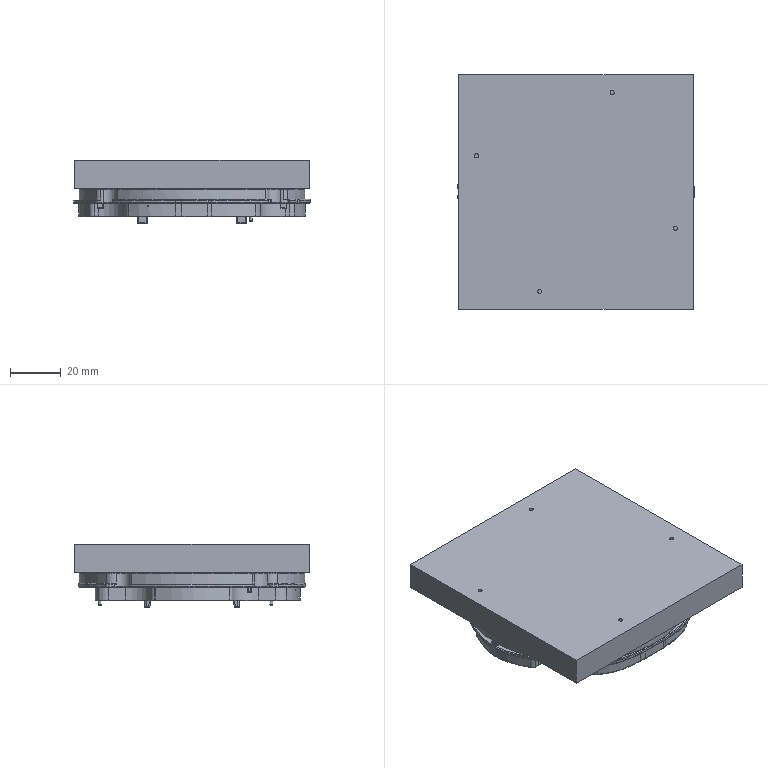NC program | NX | posted with a generic post | part box 92.935 x 92.1 x 24.829 mm
Lines 5782 to 7422 of 7643, first 1500 of 1619 lines:
(PLANAR_MILL_2_COPY , TOOL : D8-25-D8-60-3T-FINISH)
N11508 T16 M6
N11510 G53
N11512 G17 G0 G90 X-29.055 Y-31.838 S3500 M3
N11514 G43 Z21. H16
N11516 Z2.
N11518 G94 G1 Z0. F800.
N11520 G3 X-29.055 Y-29.009 R2.
N11522 G1 X-44.744 Y-13.321
N11524 G2 X-47.69 Y-7.539 R10.5
N11526 X-47.69 Y7.563 R48.25
N11528 X-44.744 Y13.345 R10.5
N11530 G1 X-13.367 Y44.721
N11532 G2 X-7.586 Y47.667 R10.5
N11534 X7.517 Y47.667 R48.25
N11536 X13.298 Y44.721 R10.5
N11538 G1 X18.008 Y40.012
N11540 X23.489
N11542 G2 X30.689 Y32.812 R7.2
N11544 G1 Y27.331
N11546 X44.675 Y13.345
N11548 G2 X47.621 Y7.563 R10.5
N11550 X47.621 Y-7.539 R48.25
N11552 X44.675 Y-13.321 R10.5
N11554 G1 X13.298 Y-44.697
N11556 G2 X7.517 Y-47.643 R10.5
N11558 X-7.586 Y-47.643 R48.25
N11560 X-13.367 Y-44.697 R10.5
N11562 G1 X-29.055 Y-29.009
N11564 G3 X-31.884 Y-29.009 R2.
N11566 G1 X-26.793 Y-29.575
N11568 G3 X-26.793 Y-26.746 R2.
N11570 G1 X-42.481 Y-11.058
N11572 G2 X-44.529 Y-7.039 R7.3
N11574 X-44.529 Y7.063 R45.05
N11576 X-42.481 Y11.082 R7.3
N11578 G1 X-11.104 Y42.459
N11580 G2 X-7.085 Y44.507 R7.3
N11582 X7.016 Y44.507 R45.05
N11584 X11.036 Y42.459 R7.3
N11586 G1 X15.892 Y37.603
N11588 G3 X17.801 Y36.812 R2.7
N11590 G1 X23.489
N11592 G2 X27.489 Y32.812 R4.
N11594 G1 Y27.124
N11596 G3 X28.279 Y25.215 R2.7
N11598 G1 X42.412 Y11.082
N11600 G2 X44.461 Y7.063 R7.3
N11602 X44.461 Y-7.039 R45.05
N11604 X42.412 Y-11.058 R7.3
N11606 G1 X11.036 Y-42.435
N11608 G2 X7.016 Y-44.483 R7.3
N11610 X-7.085 Y-44.483 R45.05
N11612 X-11.104 Y-42.435 R7.3
N11614 G1 X-26.793 Y-26.746
N11616 G3 X-29.621 Y-26.746 R2.
N11618 G1 X-31.884 Y-29.009
N11620 Z2.
N11622 G0 Z21.
(CAVITY_MILL , TOOL : D8-25-D8-60-3T-FINISH)
N11624 X1.671 Y-50.455
N11626 Z-14.
N11628 G1 Z-16.
N11630 G3 X-0.324 Y-48.45 R2.
N11632 G2 X-4.38 Y-48.368 R115.196
N11634 X-10.048 Y-48.015 R114.29
N11636 X-16.205 Y-47.161 R61.388
N11638 X-32.308 Y-38.078 R28.936
N11640 G1 X-33.519 Y-36.693
N11642 X-33.793 Y-36.363
N11644 G2 X-33.961 Y-28.359 R6.5
N11646 X-41.317 Y-25.28 R6.5
N11648 X-43.941 Y-20.593 R129.164
N11650 X-46.464 Y-15.535 R114.943
N11652 X-48.477 Y-10.777 R68.598
N11654 X-50.456 Y-2.103 R32.214
N11656 X-50.073 Y0.011 R4.3
N11658 X-50.454 Y2.154 R4.3
N11660 X-48.523 Y10.684 R31.993
N11662 X-46.592 Y15.285 R66.496
N11664 X-45.02 Y18.536 R112.281
N11666 X-41.353 Y25.25 R129.675
N11668 X-33.963 Y28.384 R6.5
N11670 X-33.705 Y36.509 R6.5
N11672 X-28.545 Y41.616 R34.394
N11674 X-16.607 Y47.104 R28.827
N11676 X-10.678 Y47.982 R55.54
N11678 X-6.588 Y48.287 R111.688
N11680 X-2.445 Y48.449 R115.301
N11682 X-1.044 Y48.251 R4.3
N11684 X0.972 Y48.251 R48.25
N11686 X2.355 Y48.449 R4.3
N11688 X4.104 Y48.399 R114.744
N11690 X9.678 Y48.065 R114.29
N11692 X15.539 Y47.305 R66.535
N11694 X26.538 Y43.003 R29.794
N11696 X33.703 Y36.414 R31.821
N11698 X33.892 Y28.383 R6.5
N11700 X41.261 Y25.285 R6.5
N11702 X43.797 Y20.757 R141.665
N11704 X46.421 Y15.505 R114.366
N11706 X48.547 Y10.423 R66.341
N11708 X50.467 Y0.009 R30.866
N11710 X48.795 Y-9.687 R30.272
N11712 X46.793 Y-14.676 R56.558
N11714 X44.979 Y-18.453 R112.279
N11716 X41.573 Y-24.733 R115.6
N11718 X41.217 Y-25.345 R1481.554
N11720 X33.893 Y-28.36 R6.5
N11722 X33.709 Y-36.385 R6.5
N11724 X32.19 Y-38.147 R44.69
N11726 X24.473 Y-44.21 R29.481
N11728 X15.568 Y-47.276 R30.376
N11730 X10.062 Y-48.007 R63.2
N11732 X6.545 Y-48.262 R111.688
N11734 X-0.324 Y-48.45 R115.196
N11736 G3 X-2.329 Y-50.445 R2.
N11738 G1 X1.671 Y-50.455
N11740 G3 X-0.324 Y-48.45 R2.
N11742 G2 X-4.38 Y-48.368 R115.196
N11744 X-10.048 Y-48.015 R114.29
N11746 X-16.205 Y-47.161 R61.388
N11748 X-32.308 Y-38.078 R28.936
N11750 G1 X-33.519 Y-36.693
N11752 X-33.793 Y-36.363
N11754 G2 X-33.961 Y-28.359 R6.5
N11756 X-41.317 Y-25.28 R6.5
N11758 X-43.941 Y-20.593 R129.164
N11760 X-46.464 Y-15.535 R114.943
N11762 X-48.477 Y-10.777 R68.598
N11764 X-50.456 Y-2.103 R32.214
N11766 X-50.073 Y0.011 R4.3
N11768 X-50.454 Y2.154 R4.3
N11770 X-48.523 Y10.684 R31.993
N11772 X-46.592 Y15.285 R66.496
N11774 X-45.02 Y18.536 R112.281
N11776 X-41.353 Y25.25 R129.675
N11778 X-33.963 Y28.384 R6.5
N11780 X-33.705 Y36.509 R6.5
N11782 X-28.545 Y41.616 R34.394
N11784 X-16.607 Y47.104 R28.827
N11786 X-10.678 Y47.982 R55.54
N11788 X-6.588 Y48.287 R111.688
N11790 X-2.445 Y48.449 R115.301
N11792 X-1.044 Y48.251 R4.3
N11794 X0.972 Y48.251 R48.25
N11796 X2.355 Y48.449 R4.3
N11798 X4.104 Y48.399 R114.744
N11800 X9.678 Y48.065 R114.29
N11802 X15.539 Y47.305 R66.535
N11804 X26.538 Y43.003 R29.794
N11806 X33.703 Y36.414 R31.821
N11808 X33.892 Y28.383 R6.5
N11810 X41.261 Y25.285 R6.5
N11812 X43.797 Y20.757 R141.665
N11814 X46.421 Y15.505 R114.366
N11816 X48.547 Y10.423 R66.341
N11818 X50.467 Y0.009 R30.866
N11820 X48.795 Y-9.687 R30.272
N11822 X46.793 Y-14.676 R56.558
N11824 X44.979 Y-18.453 R112.279
N11826 X41.573 Y-24.733 R115.6
N11828 X41.217 Y-25.345 R1481.554
N11830 X33.893 Y-28.36 R6.5
N11832 X33.709 Y-36.385 R6.5
N11834 X32.19 Y-38.147 R44.69
N11836 X24.473 Y-44.21 R29.481
N11838 X15.568 Y-47.276 R30.376
N11840 X10.062 Y-48.007 R63.2
N11842 X6.545 Y-48.262 R111.688
N11844 X-0.324 Y-48.45 R115.196
N11846 G3 X-2.329 Y-50.445 R2.
N11848 G1 Z-14.
N11850 G0 Z21.
(PLANAR_MILL_2 , TOOL : D8-25-D8-60-3T-FINISH)
N11852 X-2.034 Y50.262
N11854 Z-2.303
N11856 G1 Z-4.303
N11858 G3 X-0.034 Y48.262 R2.
N11860 G2 X31.651 Y36.4 R48.25
N11862 X33.65 Y28.312 R7.25
N11864 X36.623 Y28.526 R6.5
N11866 X40.74 Y25.81 R6.
N11868 X40.738 Y-25.788 R48.25
N11870 X36.572 Y-28.512 R6.
N11872 X33.65 Y-28.289 R6.5
N11874 X31.651 Y-36.376 R7.25
N11876 X-31.719 Y-36.376 R48.25
N11878 X-33.718 Y-28.288 R7.25
N11880 X-36.719 Y-28.497 R6.5
N11882 X-40.809 Y-25.785 R6.
N11884 X-40.807 Y25.813 R48.25
N11886 X-36.633 Y28.537 R6.
N11888 X-33.718 Y28.313 R6.5
N11890 X-31.719 Y36.4 R7.25
N11892 X-0.034 Y48.262 R48.25
N11894 G3 X1.966 Y50.262 R2.
N11896 G1 Z-2.303
N11898 G0 Z21.
(PLANAR_MILL_2_COPY_1 , TOOL : D8-25-D8-60-3T-FINISH)
N11900 X-35.896 Y-29.647
N11902 Z-2.603
N11904 G1 Z-4.603
N11906 G3 X-36.719 Y-28.497 R1.
N11908 G2 X-40.809 Y-25.785 R6.
N11910 X-40.807 Y25.813 R48.25
N11912 X-36.633 Y28.537 R6.
N11914 G3 X-35.793 Y29.675 R1.
N11916 G1 Z-2.603
N11918 G0 Z21.
(FLOOR_FACING , TOOL : D8-25-D8-60-3T-FINISH)
N11920 X-0.047 Y-5.126
N11922 Z-0.053
N11924 G1 X-0.034 Y-5.139 Z-0.057
N11926 X1.155 Y-3.95 Z-0.353
N11928 X0.997 Y-2.863 Z-0.547
N11930 X0.926 Y-1.768 Z-0.74
N11932 X-0.216 Y-1.174 Z-0.967
N11934 X-0.458 Y-1.031 Z-1.017
N11936 X-2.832 Y0.553 Z-1.52
N11938 X-3.828 Y1.369 Z-1.747
N11940 X-5.185 Y0.012 Z-2.085
N11942 X-0.034 Y-5.139 Z-3.37
N11944 X1.155 Y-3.95 Z-3.666
N11946 X0.997 Y-2.863 Z-3.86
N11948 X0.926 Y-1.768 Z-4.053
N11950 G2 X-3.828 Y1.369 R27.6
N11952 G1 X-5.185 Y0.012
N11954 X-0.034 Y-5.139
N11956 X1.155 Y-3.95
N11958 G2 X0.926 Y-1.768 R27.6
N11960 G1 X4.469 Y0.548
N11962 G2 X-3.912 Y6.376 R24.
N11964 G1 X-10.276 Y0.012
N11966 X-0.034 Y-10.23
N11968 X5.033 Y-5.162
N11970 G2 X4.469 Y0.015 R24.
N11972 G1 Y0.548
N11974 X10.469 Y5.001
N11976 G2 X-2.957 Y15.816 R18.
N11978 G1 X-18.761 Y0.012
N11980 X-0.034 Y-18.715
N11982 X11.829 Y-6.851
N11984 G2 X10.469 Y0.015 R18.
N11986 G1 Y5.001
N11988 X6.823 Y12.858
N11990 G2 X1.669 Y22.715 R12.
N11992 G1 Y25.521
N11994 X0.739 Y26.451
N11996 G3 X-0.808 Y26.451 R26.45
N11998 G1 X-26.473 Y0.786
N12000 G3 X-26.473 Y-0.762 R26.45
N12002 G1 X-0.808 Y-26.427
N12004 G3 X0.739 Y-26.427 R26.45
N12006 G1 X19.364 Y-7.802
N12008 G2 X16.469 Y0.015 R12.
N12010 G1 Y10.715
N12012 X13.669
N12014 G2 X6.823 Y12.858 R12.
N12016 G1 X13.669 Y16.715
N12018 G2 X7.669 Y22.715 R6.
N12020 G1 Y28.048
N12022 G2 X6.982 Y28.693 R15.3
N12024 G1 X3.395 Y32.28
N12026 G3 X-3.464 Y32.28 R32.45
N12028 G1 X-32.303 Y3.441
N12030 G3 X-32.303 Y-3.417 R32.45
N12032 G1 X-3.464 Y-32.256
N12034 G3 X3.395 Y-32.256 R32.45
N12036 G1 X29.666 Y-5.985
N12038 X33.681 Y-4.32
N12040 X29.666 Y-5.985
N12042 X28.469
N12044 G2 X22.469 Y0.015 R6.
N12046 G1 Y13.207
N12048 X19.37 Y16.305
N12050 G2 X18.976 Y16.715 R15.3
N12052 G1 X13.669
N12054 Y22.715
N12056 Y31.18
N12058 G2 X11.225 Y32.936 R9.3
N12060 G1 X6.369 Y37.792
N12062 G3 X5.983 Y37.988 R0.7
N12064 X-6.052 Y37.988 R38.45
N12066 X-6.437 Y37.792 R0.7
N12068 G1 X-37.814 Y6.415
N12070 G3 X-38.01 Y6.03 R0.7
N12072 X-38.01 Y-6.006 R38.45
N12074 X-37.814 Y-6.391 R0.7
N12076 G1 X-6.437 Y-37.768
N12078 G3 X-6.052 Y-37.964 R0.7
N12080 X5.983 Y-37.964 R38.45
N12082 X6.369 Y-37.768 R0.7
N12084 G1 X37.746 Y-6.391
N12086 G3 X37.942 Y-6.006 R0.7
N12088 X38.416 Y0.015 R38.45
N12090 G1 X28.469
N12092 Y14.009
N12094 X30.151
N12096 X23.613 Y20.548
N12098 G2 X22.001 Y22.715 R9.3
N12100 G1 X13.669
N12102 Y23.715
N12104 G2 X15.669 Y25.715 R2.
N12106 G1 Z-1.053
N12108 G0 Z21.
N12110 M5
(PLANAR_MILL_3 , TOOL : D3R0.2)
N12112 T17 M6
N12114 G53
N12116 G17 G0 G90 X-24.106 Y-21.231 S3500 M3
N12118 G43 Z21. H17
N12120 Z-2.053
N12122 G94 G1 Z-4.053 F600.
N12124 G3 X-24.106 Y-24.059 R2.
N12126 G1 X-8.417 Y-39.748
N12128 G3 X-6.49 Y-40.73 R3.5
N12130 X6.422 Y-40.73 R41.25
N12132 X8.349 Y-39.748 R3.5
N12134 G1 X39.725 Y-8.371
N12136 G3 X40.707 Y-6.444 R3.5
N12138 X40.707 Y6.468 R41.25
N12140 X39.725 Y8.395 R3.5
N12142 G1 X25.592 Y22.528
N12144 G2 X23.689 Y27.124 R6.5
N12146 G1 Y33.012
N12148 X17.801
N12150 G2 X13.205 Y34.916 R6.5
N12152 G1 X8.349 Y39.772
N12154 G3 X6.422 Y40.754 R3.5
N12156 X-6.49 Y40.754 R41.25
N12158 X-8.417 Y39.772 R3.5
N12160 G1 X-39.794 Y8.395
N12162 G3 X-40.776 Y6.468 R3.5
N12164 X-40.776 Y-6.444 R41.25
N12166 X-39.794 Y-8.371 R3.5
N12168 G1 X-24.106 Y-24.059
N12170 G3 X-21.277 Y-24.059 R2.
N12172 G1 X-24.106 Y-21.231
N12174 G3 X-24.106 Y-24.059 R2.
N12176 G1 X-8.417 Y-39.748
N12178 G3 X-6.49 Y-40.73 R3.5
N12180 X6.422 Y-40.73 R41.25
N12182 X8.349 Y-39.748 R3.5
N12184 G1 X39.725 Y-8.371
N12186 G3 X40.707 Y-6.444 R3.5
N12188 X40.707 Y6.468 R41.25
N12190 X39.725 Y8.395 R3.5
N12192 G1 X25.592 Y22.528
N12194 G2 X23.689 Y27.124 R6.5
N12196 G1 Y33.012
N12198 X17.801
N12200 G2 X13.205 Y34.916 R6.5
N12202 G1 X8.349 Y39.772
N12204 G3 X6.422 Y40.754 R3.5
N12206 X-6.49 Y40.754 R41.25
N12208 X-8.417 Y39.772 R3.5
N12210 G1 X-39.794 Y8.395
N12212 G3 X-40.776 Y6.468 R3.5
N12214 X-40.776 Y-6.444 R41.25
N12216 X-39.794 Y-8.371 R3.5
N12218 G1 X-24.106 Y-24.059
N12220 G3 X-21.277 Y-24.059 R2.
N12222 G1 Z-2.053
N12224 G0 Z21.
N12226 M5
(PLANAR_MILL_13 , TOOL : D3NEIR0.5)
N12228 T18 M6
N12230 G53
N12232 G17 G0 G90 X-0.947 Y46.954 S3500 M3
N12234 G43 Z21. H18
N12236 Z1.7
N12238 G94 G1 Z-0.3 F800.
N12240 G41 X-1.034 Y46.462 D18
N12242 G3 X-0.034 Y45.462 R1.
N12244 G2 X29.812 Y34.289 R45.45
N12246 X30.929 Y29.065 R4.45
N12248 G3 X34.238 Y25.553 R2.6
N12250 G2 X36.178 Y25.762 R3.7
N12252 X38.373 Y24.313 R3.2
N12254 X38.372 Y-24.291 R45.45
N12256 X36.15 Y-25.744 R3.2
N12258 X34.24 Y-25.529 R3.7
N12260 G3 X30.929 Y-29.041 R2.6
N12262 G2 X29.812 Y-34.265 R4.45
N12264 X-29.881 Y-34.265 R45.45
N12266 X-30.997 Y-29.041 R4.45
N12268 G3 X-34.306 Y-25.529 R2.6
N12270 G2 X-36.262 Y-25.734 R3.7
N12272 X-38.443 Y-24.288 R3.2
N12274 X-38.441 Y24.315 R45.45
N12276 X-36.215 Y25.768 R3.2
N12278 X-34.308 Y25.553 R3.7
N12280 G3 X-30.997 Y29.065 R2.6
N12282 G2 X-29.881 Y34.289 R4.45
N12284 X-0.034 Y45.462 R45.45
N12286 G3 X0.966 Y46.462 R1.
N12288 G40
N12290 G1 X0.879 Y46.954
N12292 Z1.7
N12294 G0 Z21.
(PLANAR_MILL_13_COPY , TOOL : D3NEIR0.5)
N12296 X-23.908 Y-22.57
N12298 Z1.7
N12300 G1 Z-0.3
N12302 G41 X-24.318 Y-22.857
N12304 G3 X-24.318 Y-24.271 R1.
N12306 G1 X-8.629 Y-39.96
N12308 G3 X-6.537 Y-41.026 R3.8
N12310 X6.469 Y-41.026 R41.55
N12312 X8.561 Y-39.96 R3.8
N12314 G1 X39.938 Y-8.583
N12316 G3 X41.004 Y-6.491 R3.8
N12318 X41.004 Y6.515 R41.55
N12320 X39.938 Y8.607 R3.8
N12322 G1 X25.805 Y22.74
N12324 G2 X23.989 Y27.124 R6.2
N12326 G1 Y33.012
N12328 G3 X23.689 Y33.312 R0.3
N12330 G1 X17.801
N12332 G2 X13.417 Y35.128 R6.2
N12334 G1 X8.561 Y39.984
N12336 G3 X6.469 Y41.05 R3.8
N12338 X-6.537 Y41.05 R41.55
N12340 X-8.629 Y39.984 R3.8
N12342 G1 X-40.006 Y8.607
N12344 G3 X-41.072 Y6.515 R3.8
N12346 X-41.072 Y-6.491 R41.55
N12348 X-40.006 Y-8.583 R3.8
N12350 G1 X-24.318 Y-24.271
N12352 G3 X-22.903 Y-24.271 R1.
N12354 G40
N12356 G1 X-22.617 Y-23.862
N12358 Z1.7
N12360 G0 Z21.
N12362 M5
(PLANAR_MILL_14 , TOOL : 倒角D4-90度)
N12364 T11 M6
N12366 G53
N12368 G17 G0 G90 X-34.955 Y-20.104 S3500 M3
N12370 G43 Z21. H11
N12372 Z1.
N12374 G94 G1 Z-1. F300.
N12376 G41 X-34.758 Y-20.138 D11
N12378 X-34.738
N12380 G3 X-34.538 Y-19.938 R0.2
N12382 X-35.738 Y-18.738 R1.2
N12384 X-34.538 Y-19.938 R-1.2
N12386 X-34.758 Y-19.738 R0.201
N12388 G40
N12390 G1 X-34.955 Y-19.773
N12392 Z1.
N12394 G0 Z21.
N12396 Y19.797
N12398 Z1.
N12400 G1 Z-1.
N12402 G41 X-34.758 Y19.762
N12404 X-34.738
N12406 G3 X-34.538 Y19.962 R0.2
N12408 X-35.738 Y21.162 R1.2
N12410 X-34.538 Y19.962 R-1.2
N12412 X-34.758 Y20.162 R0.201
N12414 G40
N12416 G1 X-34.955 Y20.128
N12418 Z1.
N12420 G0 Z21.
N12422 X36.452 Y19.797
N12424 Z1.
N12426 G1 Z-1.
N12428 G41 X36.649 Y19.762
N12430 X36.669
N12432 G3 X36.869 Y19.962 R0.2
N12434 X35.669 Y21.162 R1.2
N12436 X36.869 Y19.962 R-1.2
N12438 X36.649 Y20.162 R0.201
N12440 G40
N12442 G1 X36.452 Y20.128
N12444 Z1.
N12446 G0 Z21.
N12448 Y-20.104
N12450 Z1.
N12452 G1 Z-1.
N12454 G41 X36.649 Y-20.138
N12456 X36.669
N12458 G3 X36.869 Y-19.938 R0.2
N12460 X35.669 Y-18.738 R1.2
N12462 X36.869 Y-19.938 R-1.2
N12464 X36.649 Y-19.738 R0.201
N12466 G40
N12468 G1 X36.452 Y-19.773
N12470 Z1.
N12472 G0 Z21.
N12474 M5
(ZLEVEL_PROFILE_STEEP_1 , TOOL : D3R0.2)
N12476 T17 M6
N12478 G53
N12480 G17 G0 G90 X-43.535 Y-18.489 S4500 M3
N12482 G43 Z21. H17
N12484 Z-3.633
N12486 G94 G1 Z-4.633 F2000.
N12488 X-42.998 Y-18.216
N12490 G3 X-42.605 Y-17.005 R0.9
N12492 G2 X-46.216 Y-8.571 R68.826
N12494 X-47.632 Y-1.9 R31.804
N12496 X-46.167 Y-0.319 R1.469
N12498 G1 X-45.994
N12500 Y0.343
N12502 X-46.168
N12504 G2 X-47.632 Y1.923 R1.469
N12506 X-45.208 Y11.339 R33.041
N12508 G1 X-45.026 Y11.658
N12510 X-44.882 Y12.079
N12512 G2 X-42.493 Y17.157 R53.414
N12514 G1 X-42.537 Y17.184 Z-4.647
N12516 X-42.548 Y17.191 Z-4.662
N12518 G3 X-45.49 Y10.815 R67.718
N12520 X-47.699 Y1.928 R31.725
N12522 X-46.168 Y0.277 R1.535
N12524 G1 X-46.06
N12526 Y-0.253
N12528 X-46.167
N12530 G3 X-47.696 Y-1.928 R1.535
N12532 X-46.124 Y-9.043 R28.925
N12534 X-42.664 Y-17.035 R67.376
N12536 G1 X-42.668 Y-17.037 Z-4.677
N12538 X-42.708 Y-17.056 Z-4.691
N12540 G2 X-45.414 Y-11.124 R81.437
N12542 X-47.269 Y-5.183 R36.569
N12544 X-47.749 Y-1.861 R40.162
N12546 X-46.167 Y-0.204 R1.584
N12548 G1 X-46.109
N12550 Y0.228
N12552 X-46.168
N12554 G2 X-47.747 Y1.932 R1.584
N12556 X-45.863 Y9.972 R30.54
N12558 X-42.6 Y17.225 R68.157
N12560 G1 X-42.65 Y17.258 Z-4.721
N12562 G3 X-44.796 Y12.705 R80.865
N12564 G1 X-44.894 Y12.501
N12566 G3 X-46.978 Y6.601 R40.727
N12568 X-47.785 Y1.935 R29.888
N12570 X-46.147 Y0.19 R1.622
N12572 G1 Y-0.166
N12574 X-46.167
N12576 G3 X-47.785 Y-1.912 R1.622
N12578 X-46.105 Y-9.414 R31.006
N12580 X-42.742 Y-17.074 R70.169
N12582 G1 X-42.737 Y-17.071 Z-4.736
N12584 X-42.771 Y-17.088 Z-4.75
N12586 G2 X-45.62 Y-10.824 R83.467
N12588 X-47.574 Y-3.935 R34.633
N12590 X-47.819 Y-1.868 R103.283
N12592 X-46.179 Y-0.134 R1.654
N12594 G1 Y0.158
N12596 G2 X-47.817 Y1.937 R1.654
N12598 X-46.445 Y8.536 R30.427
N12600 X-44.373 Y13.765 R53.148
N12602 G1 X-44.221 Y14.08
N12604 X-43.982 Y14.608
N12606 X-42.68 Y17.282
N12608 X-42.702 Y17.3 Z-4.78
N12610 G3 X-46.134 Y9.551 R71.483
N12612 X-47.844 Y1.94 R30.68
N12614 X-46.206 Y0.131 R1.681
N12616 G1 Y-0.107
N12618 G3 X-47.843 Y-1.917 R1.681
N12620 X-46.032 Y-9.809 R30.477
N12622 X-42.795 Y-17.1 R71.978
N12624 G1 X-42.815 Y-17.111 Z-4.809
N12626 G2 X-45.889 Y-10.256 R74.252
N12628 X-47.866 Y-1.918 R30.729
N12630 X-46.229 Y-0.085 R1.704
N12632 G1 Y0.109
N12634 G2 X-47.867 Y1.941 R1.704
N12636 X-45.848 Y10.393 R30.486
N12638 X-42.722 Y17.317 R78.063
N12640 G1 X-42.745 Y17.321 Z-4.838
N12642 G3 X-45.873 Y10.393 R79.63
N12644 X-47.887 Y1.943 R30.56
N12646 X-46.249 Y0.09 R1.724
N12648 G1 Y-0.066
N12650 G3 X-47.889 Y-1.871 R1.724
N12652 X-45.911 Y-10.256 R30.816
N12654 X-42.833 Y-17.119 R75.061
N12656 G1 X-42.848 Y-17.127 Z-4.868
N12658 G2 X-45.774 Y-10.678 R79.737
N12660 X-47.428 Y-5.199 R36.332
N12662 X-47.903 Y-1.921 R30.369
N12664 X-46.266 Y-0.05 R1.741
N12666 G1 Y0.074
N12668 G2 X-47.904 Y1.944 R1.741
N12670 X-46.042 Y9.972 R29.928
N12672 G1 X-46.032 Y10.021
N12674 G2 X-43.084 Y16.671 R73.65
N12676 G1 X-43.051 Y16.715
N12678 X-42.768 Y17.302
N12680 X-42.789 Y17.282 Z-4.897
N12682 G3 X-44.082 Y14.608 R81.426
N12684 G1 X-44.277 Y14.186
N12686 X-44.32 Y14.126
N12688 G3 X-46.641 Y8.286 R51.575
N12690 X-47.918 Y1.945 R29.743
N12692 X-46.281 Y0.06 R1.756
N12694 G1 Y-0.036
N12696 G3 X-47.918 Y-1.922 R1.756
N12698 G1 X-47.681 Y-3.892
N12700 X-47.606 Y-4.356
N12702 G3 X-46.032 Y-10.03 R34.956
N12704 X-42.861 Y-17.134 R73.61
N12706 G1 X-42.872 Y-17.139 Z-4.927
N12708 G2 X-45.62 Y-11.125 R82.753
N12710 X-47.681 Y-3.978 R35.558
N12712 G1 X-47.93 Y-1.923
N12714 G2 X-46.293 Y-0.025 R1.768
N12716 G1 Y0.049
N12718 G2 X-47.93 Y1.946 R1.768
N12720 X-46.226 Y9.551 R30.871
N12722 G1 X-46.061 Y9.972
N12724 X-46.032 Y10.097
N12726 X-45.904 Y10.393
N12728 X-45.757 Y10.815
N12730 G2 X-43.504 Y15.872 R88.856
N12732 G1 X-43.282 Y16.293
N12734 X-42.809 Y17.262
N12736 X-42.828 Y17.241 Z-4.956
N12738 X-43.971 Y14.913
N12740 X-44.103 Y14.608
N12742 X-44.299 Y14.186
N12744 G3 X-46.032 Y10.115 R55.377
N12746 G1 X-46.071 Y9.972
N12748 X-46.235 Y9.551
N12750 G3 X-47.94 Y1.947 R30.692
N12752 X-46.303 Y0.039 R1.778
N12754 G1 Y-0.015
N12756 G3 X-47.94 Y-1.924 R1.778
N12758 G1 X-47.681 Y-4.046
N12760 G3 X-45.62 Y-11.145 R35.119
N12762 X-42.881 Y-17.144 R84.344
N12764 G1 X-42.889 Y-17.147 Z-4.985
N12766 G2 X-46.13 Y-9.835 R75.418
N12768 X-47.948 Y-1.925 R30.551
N12770 X-46.311 Y-0.008 R1.786
N12772 G1 Y0.032
N12774 G2 X-47.948 Y1.947 R1.786
N12776 X-46.244 Y9.551 R30.436
N12778 X-43.519 Y15.872 R64.218
N12780 G1 X-43.304 Y16.293
N12782 X-43.219 Y16.479
N12784 X-42.847 Y17.22
N12786 X-42.867 Y17.2 Z-5.015
N12788 X-43.107 Y16.715
N12790 X-43.123 Y16.693
N12792 G3 X-46.032 Y10.15 R69.624
N12794 X-47.955 Y1.948 R30.735
N12796 X-46.317 Y0.026 R1.792
N12798 G1 Y-0.002
N12800 G3 X-47.954 Y-1.925 R1.792
N12802 X-46.032 Y-10.128 R30.797
N12804 X-42.894 Y-17.15 R77.893
N12806 G1 X-42.898 Y-17.152 Z-5.044
N12808 G2 X-46.032 Y-10.145 R76.523
N12810 X-47.958 Y-1.925 R30.705
N12812 X-46.321 Y0.002 R1.796
N12814 G1 Y0.022
N12816 G2 X-47.959 Y1.948 R1.796
N12818 X-46.032 Y10.168 R30.391
N12820 X-42.887 Y17.179 R74.743
N12822 G1 X-42.907 Y17.159 Z-5.073
N12824 G3 X-46.032 Y10.186 R74.913
N12826 X-47.962 Y1.948 R30.006
N12828 X-46.324 Y0.02 R1.799
N12830 G1 Y0.004
N12832 G3 X-47.961 Y-1.926 R1.799
N12834 X-46.032 Y-10.162 R30.256
N12836 X-42.9 Y-17.153 R73.517
N12838 G1 X-42.901 Z-5.103
N12840 X-43.143 Y-16.666
N12842 X-43.382 Y-16.183
N12844 X-43.813 Y-15.294
N12846 X-44.401 Y-14.049
N12848 X-44.793 Y-13.185
N12850 X-45.508 Y-11.511
N12852 X-45.831 Y-10.705
N12854 X-46.166 Y-9.82
N12856 X-46.445 Y-9.026
N12858 X-46.731 Y-8.149
N12860 X-46.981 Y-7.291
N12862 X-47.204 Y-6.464
N12864 X-47.494 Y-5.185
N12866 X-47.681 Y-4.199
N12868 X-47.853 Y-3.005
N12870 X-47.923 Y-2.336
N12872 X-47.967 Y-1.784
N12874 G2 X-47.778 Y-0.985 R1.8
N12876 G1 X-47.681 Y-0.815
N12878 X-47.59 Y-0.685
N12880 X-47.422 Y-0.498
N12882 X-47.382 Y-0.46
N12884 G2 X-46.823 Y-0.112 R1.8
N12886 X-46.512 Y-0.021 R1.8
N12888 G1 X-46.341 Y0.004
N12890 X-46.325 Y0.019
N12892 X-46.331
N12894 X-46.393 Y0.026
N12896 G2 X-46.719 Y0.098 R1.8
N12898 G1 X-47.014 Y0.224
N12900 X-47.152 Y0.305
N12902 G2 X-47.965 Y1.914 R1.8
N12904 G1 X-47.958 Y1.994
N12906 G2 X-47.681 Y4.227 R26.866
N12908 G1 X-47.558 Y4.915
N12910 X-47.375 Y5.795
N12912 X-46.952 Y7.443
N12914 X-46.857 Y7.769
N12916 X-46.432 Y9.095
N12918 X-46.279 Y9.538
N12920 X-45.444 Y11.694
N12922 X-44.92 Y12.922
N12924 X-44.797 Y13.198
N12926 X-44.731 Y13.343
N12928 X-44.341 Y14.199
N12930 X-43.95 Y15.029
N12932 X-43.741 Y15.468
N12934 X-43.347 Y16.278
N12936 X-43.195 Y16.59
N12938 X-43.147 Y16.689
N12940 X-42.923 Y17.137
N12942 G3 X-43.325 Y18.344 R0.9
N12944 G1 X-43.856 Y18.609
N12946 Z-4.103
N12948 G0 Z21.
(ZLEVEL_PROFILE_STEEP_1_COPY , TOOL : D3R0.2)
N12950 X-32.832 Y28.797
N12952 Z-3.333
N12954 G1 Z-4.333
N12956 X-32.308 Y28.905
N12958 G3 X-31.61 Y29.969 R0.9
N12960 G2 X-31.555 Y34.668 R3.669
N12962 X-24.913 Y40.708 R32.042
N12964 X-14.241 Y44.643 R27.712
N12966 G1 X-12.246 Y44.937
N12968 X-6.757 Y45.429
N12970 X-6.628 Y45.425
N12972 X-6.503 Y45.501 Z-4.362
N12974 X-9.29 Y45.302
N12976 G3 X-17.066 Y44.126 R47.457
N12978 X-28.939 Y37.562 R25.263
N12980 X-31.605 Y34.711 R46.437
N12982 X-31.578 Y29.829 R3.735
N12984 G1 X-31.553 Y29.729 Z-4.392
N12986 G2 X-31.642 Y34.743 R3.784
N12988 X-27.446 Y38.999 R39.587
N12990 X-16.046 Y44.424 R26.283
N12992 X-8.868 Y45.395 R54.923
N12994 G1 X-8.446 Y45.407
N12996 X-6.429 Y45.57
N12998 X-6.454 Y45.602 Z-4.421
N13000 X-6.757 Y45.586
N13002 X-8.446 Y45.445
N13004 X-8.868 Y45.439
N13006 G3 X-11.401 Y45.189 R47.474
N13008 X-18.157 Y43.928 R37.569
N13010 X-29.557 Y37.099 R25.583
N13012 G1 X-29.976 Y36.661
N13014 X-31.671 Y34.768
N13016 G3 X-31.551 Y29.669 R3.822
N13018 G1 X-31.558 Y29.663 Z-4.436
N13020 X-31.574 Y29.647 Z-4.45
N13022 G2 X-31.695 Y34.788 R3.854
N13024 X-29.557 Y37.141 R66.149
N13026 X-18.157 Y43.965 R25.519
N13028 X-15.624 Y44.604 R55.657
N13030 X-9.712 Y45.398 R59.046
N13032 X-6.478 Y45.634 R136.14
N13034 G1 X-6.503 Y45.665 Z-4.48
N13036 G3 X-11.401 Y45.257 R100.948
N13038 G1 X-11.824 Y45.208
N13040 X-12.246 Y45.165
N13042 G3 X-17.735 Y44.112 R37.497
N13044 X-29.557 Y37.182 R25.566
N13046 X-31.716 Y34.806 R57.906
N13048 X-31.594 Y29.629 R3.881
N13050 G1 X-31.603 Y29.62 Z-4.509
N13052 G2 X-31.726 Y34.814 R3.894
N13054 X-29.557 Y37.205 R58.372
N13056 X-17.735 Y44.127 R25.596
N13058 X-12.668 Y45.127 R36.574
N13060 X-6.515 Y45.678 R97.075
N13062 G1 X-6.55 Y45.703 Z-4.539
N13064 G3 X-13.151 Y45.083 R85.183
N13066 X-18.352 Y43.988 R35.487
N13068 X-28.625 Y38.143 R25.395
N13070 X-31.749 Y34.834 R36.634
N13072 X-31.625 Y29.6 R3.924
N13074 G1 X-31.638 Y29.588 Z-4.568
N13076 G2 X-31.762 Y34.845 R3.941
N13078 X-28.749 Y38.052 R37.762
N13080 X-18.326 Y44.015 R25.388
N13082 X-12.246 Y45.222 R36.603
N13084 X-6.573 Y45.719 R101.476
N13086 G1 X-6.595 Y45.73 Z-4.597
N13088 G3 X-12.449 Y45.21 R102.94
N13090 X-18.189 Y44.066 R36.853
N13092 X-28.713 Y38.103 R25.511
N13094 X-31.772 Y34.854 R37.385
N13096 X-31.648 Y29.578 R3.955
N13098 G1 X-31.657 Y29.57 Z-4.627
N13100 G2 X-31.782 Y34.862 R3.968
N13102 X-28.916 Y37.932 R43.772
N13104 X-18.157 Y44.085 R25.634
N13106 X-13.09 Y45.142 R36.055
N13108 X-6.619 Y45.737 R99.989
N13110 G1 X-6.642 Y45.744 Z-4.656
N13112 G3 X-13.09 Y45.149 R95.335
N13114 X-16.89 Y44.438 R40.341
N13116 G1 X-17.313 Y44.323
N13118 X-17.478 Y44.288
N13120 G3 X-23.818 Y41.746 R27.033
N13122 X-30.402 Y36.432 R27.305
N13124 G2 X-31.79 Y34.869 R230.82
N13126 G3 X-31.664 Y29.563 R3.978
N13128 G1 X-31.67 Y29.557 Z-4.686
N13130 G2 X-31.796 Y34.874 R3.986
N13132 X-29.795 Y37.085 R107.323
N13134 X-17.313 Y44.333 R25.878
N13136 X-12.668 Y45.212 R37.184
N13138 X-6.665 Y45.751 R95.787
N13140 G1 X-6.688 Y45.757 Z-4.715
N13142 G3 X-11.401 Y45.368 R98.447
N13144 X-17.313 Y44.343 R40.537
N13146 X-29.806 Y37.085 R25.873
N13148 G1 X-30.209 Y36.661
N13150 X-31.8 Y34.878
N13152 G3 X-31.675 Y29.553 R3.992
N13154 G1 X-31.678 Y29.55 Z-4.744
N13156 G2 X-31.804 Y34.881 R3.997
N13158 X-29.262 Y37.637 R41.167
N13160 X-16.431 Y44.566 R25.925
N13162 X-8.868 Y45.612 R52.575
N13164 G1 X-6.711 Y45.764
N13166 X-6.734 Y45.77 Z-4.774
N13168 X-8.446 Y45.656
N13170 X-10.062 Y45.519
N13172 G3 X-16.424 Y44.576 R51.29
N13174 X-28.944 Y37.954 R25.926
N13176 X-31.825 Y34.86 R36.567
N13178 X-31.68 Y29.548 R3.999
N13180 G2 X-31.72 Y28.276 R0.9
N13182 G1 X-32.571 Y28.119
N13184 Z-3.774
N13186 G0 Z21.
N13188 X-17.222 Y45.944
N13190 Z-3.803
N13192 G1 Z-4.803
N13194 X-17.106 Y45.371
N13196 G3 X-16.046 Y44.667 R0.9
N13198 G1 X-15.823 Y44.712
N13200 X-13.935 Y45.058
N13202 X-13.513 Y45.12
N13204 X-13.406 Y45.136
N13206 X-12.668 Y45.24
N13208 X-12.246 Y45.292
N13210 X-10.506 Y45.489
N13212 X-9.674 Y45.559
N13214 X-9.29 Y45.592
N13216 X-8.446 Y45.659
N13218 X-7.935 Y45.697
N13220 G3 X-7.105 Y46.662 R0.9
N13222 G1 X-7.149 Y47.252
N13224 Z-3.803
N13226 G0 Z21.
N13228 X-32.573 Y28.134
N13230 Z-3.803
N13232 G1 Z-4.803
N13234 X-31.771 Y28.298
N13236 G3 X-31.7 Y29.569 R0.9
N13238 G1 X-31.779 Y29.656
N13240 G2 X-32.744 Y32.692 R4.
N13242 G1 X-32.735 Y32.77
N13244 G2 X-31.788 Y34.904 R4.
N13246 G1 X-30.624 Y36.237
N13248 X-30.402 Y36.481
N13250 X-30.237 Y36.661
N13252 G3 X-30.294 Y37.933 R0.9
N13254 G1 X-30.726 Y38.327
N13256 Z-3.803
N13258 G0 Z21.
N13260 X-32.365 Y36.548
N13262 Z-3.833
N13264 G1 Z-4.833
N13266 X-31.909 Y36.171
N13268 G2 X-31.788 Y34.904 R0.9
N13270 G1 X-31.905 Y34.763
N13272 G3 X-32.443 Y30.715 R4.
N13274 G2 X-32.918 Y29.534 R0.9
N13276 G1 X-33.402 Y29.328
N13278 Z-3.833
N13280 G0 Z21.
N13282 X-21.62 Y44.515
N13284 Z-3.803
N13286 G1 Z-4.803
N13288 X-21.422 Y43.975
N13290 G3 X-20.268 Y43.439 R0.9
N13292 G1 X-19.846 Y43.594
N13294 X-19.424 Y43.741
N13296 X-19.005 Y43.88
N13298 X-19.017 Y43.876 Z-4.833
N13300 X-19.329 Y43.772
N13302 X-20.064 Y43.514
N13304 X-20.266 Y43.44
N13306 G2 X-21.42 Y43.976 R0.9
N13308 G1 X-21.618 Y44.517
N13310 Z-3.833
N13312 G0 Z21.
N13314 X3.616 Y47.121
N13316 Z-3.333
N13318 G1 Z-4.333
N13320 X3.591 Y46.475
N13322 G3 X4.455 Y45.541 R0.9
N13324 G2 X14.355 Y44.585 R86.067
N13326 X30.462 Y35.814 R26.258
N13328 G1 X31.528 Y34.601
N13330 G2 X31.542 Y29.971 R3.669
N13332 G1 X31.51 Y29.83 Z-4.362
N13334 G3 X31.58 Y34.643 R3.735
N13336 G1 X30.921 Y35.39
N13338 X30.821 Y35.514
N13340 G3 X21.532 Y42.597 R27.061
N13342 X12.243 Y44.995 R34.006
N13344 X4.007 Y45.636 R125.618
N13346 G1 Y45.644 Z-4.377
N13348 X4.009 Y45.685 Z-4.392
N13350 G2 X8.443 Y45.398 R145.298
N13352 G1 X8.866 Y45.391
N13354 G2 X15.621 Y44.502 R60.115
N13356 G1 X16.043 Y44.4
N13358 X16.466 Y44.323
N13360 X16.611 Y44.288
N13362 X16.888 Y44.195
N13364 X17.31 Y44.106
N13366 G2 X23.328 Y41.746 R27.367
N13368 X30.399 Y36.069 R27.213
N13370 G1 X31.617 Y34.673
N13372 G2 X31.485 Y29.729 R3.784
N13374 G1 X31.463 Y29.649 Z-4.421
N13376 G3 X31.647 Y34.698 R3.822
N13378 X29.555 Y37.008 R42.235
N13380 X20.688 Y43.043 R25.792
N13382 X16.043 Y44.453 R31.405
N13384 X8.021 Y45.468 R53.24
N13386 X4.01 Y45.723 R87.899
N13388 G1 Y45.717 Z-4.436
N13390 X4.011 Y45.755 Z-4.45
N13392 G2 X10.554 Y45.314 R155.356
N13394 X15.527 Y44.592 R51.344
N13396 X20.996 Y42.959 R29.445
N13398 X21.955 Y42.506 R9.872
N13400 X23.644 Y41.626 R12.123
N13402 X27.866 Y38.649 R21.387
N13404 X30.382 Y36.18 R24.459
N13406 G1 X31.672 Y34.718
N13408 G2 X31.503 Y29.644 R3.854
N13410 G1 X31.522 Y29.626 Z-4.48
N13412 G3 X31.692 Y34.735 R3.881
N13414 X28.722 Y37.932 R45.784
N13416 X17.732 Y44.096 R25.765
N13418 X11.821 Y45.199 R37.473
N13420 X4.012 Y45.782 R107.586
N13422 G1 X4.013 Y45.795 Z-4.509
N13424 G2 X12.666 Y45.109 R99.872
N13426 X19.87 Y43.441 R34.565
N13428 X30.006 Y36.661 R26.126
N13430 X31.703 Y34.743 R71.108
N13432 X31.532 Y29.617 R3.894
N13434 G1 X31.554 Y29.596 Z-4.539
N13436 G3 X31.726 Y34.762 R3.924
N13438 X29.555 Y37.167 R43.879
N13440 X19.959 Y43.441 R25.794
N13442 X12.666 Y45.143 R35.202
N13444 X4.014 Y45.825 R103.12
N13446 G1 X4.015 Y45.842 Z-4.568
N13448 G2 X12.837 Y45.136 R101.098
N13450 X18.577 Y43.917 R36.784
N13452 X29.245 Y37.509 R25.618
N13454 X31.739 Y34.773 R39.102
N13456 X31.566 Y29.585 R3.941
N13458 G1 X31.576 Y29.575 Z-4.597
N13460 G3 X31.75 Y34.782 R3.955
N13462 X28.912 Y37.847 R38.458
N13464 X18.644 Y43.905 R25.431
N13466 X13.917 Y44.983 R33.582
N13468 X8.081 Y45.621 R68.305
N13470 X4.015 Y45.856 R245.409
N13472 G1 X4.016 Y45.869 Z-4.627
N13474 X4.221 Y45.841
N13476 X5.488 Y45.789
N13478 G2 X12.666 Y45.174 R86.639
N13480 X20.266 Y43.367 R34.11
N13482 X29.133 Y37.646 R25.717
N13484 X31.76 Y34.79 R39.439
N13486 X31.586 Y29.567 R3.968
N13488 G1 X31.593 Y29.56 Z-4.656
N13490 G3 X31.767 Y34.796 R3.978
N13492 X28.932 Y37.855 R40.797
N13494 X19.127 Y43.767 R25.172
N13496 X12.666 Y45.185 R34.033
N13498 X5.066 Y45.816 R86.7
N13500 G1 X4.221 Y45.851
N13502 X4.016 Y45.879
N13504 Y45.887 Z-4.686
N13506 G2 X8.443 Y45.618 R328.878
N13508 X16.043 Y44.614 R54.166
N13510 X25.772 Y40.475 R26.529
N13512 X30.891 Y35.814 R29.179
N13514 G1 X31.774 Y34.801
N13516 G2 X31.599 Y29.554 R3.986
N13518 G1 X31.603 Y29.55 Z-4.715
N13520 G3 X31.778 Y34.805 R3.992
N13522 X29.555 Y37.262 R42.958
N13524 X20.266 Y43.389 R25.819
N13526 X13.088 Y45.152 R33.496
N13528 X4.016 Y45.893 R99.171
N13530 G1 X4.017 Y45.898 Z-4.744
N13532 G2 X13.51 Y45.093 R93.203
N13534 X22.148 Y42.593 R30.069
N13536 X30.148 Y36.661 R26.392
N13538 G1 X30.399 Y36.388
N13540 X31.782 Y34.808
N13542 G2 X31.607 Y29.547 R3.997
N13544 G1 X31.609 Y29.545 Z-4.774
N13546 G3 X31.784 Y34.81 R3.999
N13548 G1 X30.551 Y36.237
N13550 G3 X22.159 Y42.593 R26.551
N13552 X13.51 Y45.104 R30.017
N13554 X4.017 Y45.9 R92.183
N13556 G2 X3.146 Y46.828 R0.9
N13558 G1 X3.165 Y47.428
N13560 Z-3.774
N13562 G0 Z21.
N13564 X19.036 Y45.412
N13566 Z-3.803
N13568 G1 Z-4.803
N13570 X18.85 Y44.852
N13572 G3 X19.421 Y43.715 R0.9
N13574 G2 X21.234 Y43.017 R20.57
N13576 G1 X22.169 Y42.593
N13578 X22.377 Y42.493
N13580 X23.794 Y41.746
N13582 X24.066 Y41.589
N13584 X24.515 Y41.322
N13586 X24.91 Y41.074
N13588 X25.332 Y40.8
N13590 X25.811 Y40.475
N13592 G2 X27.444 Y39.234 R21.929
N13594 G1 X27.866 Y38.876
N13596 X28.288 Y38.503
N13598 X28.71 Y38.117
N13600 X29.555 Y37.297
N13602 X29.758 Y37.085
N13604 X30.399 Y36.409
N13606 X31.661 Y34.96
N13608 X31.824 Y34.761
N13610 G2 X32.376 Y30.729 R4.
N13612 G1 X32.341 Y30.647
N13614 G2 X31.748 Y29.7 R4.
N13616 G1 X31.707 Y29.653
N13618 X31.809 Y29.813 Z-4.813
N13620 X31.941 Y29.95 Z-4.823
N13622 X32.047 Y30.106 Z-4.833
N13624 X32.067 Y30.137
N13626 G3 X31.856 Y34.72 R4.
N13628 G1 X31.799 Y34.792
N13630 X31.824 Y34.761 Z-4.862
N13632 X31.856 Y34.72
N13634 G2 X32.047 Y30.106 R4.
N13636 G3 X32.32 Y28.862 R0.9
N13638 G1 X32.761 Y28.581
N13640 Z-3.862
N13642 G0 Z21.
N13644 X8.087 Y47.184
N13646 Z-3.803
N13648 G1 Z-4.803
N13650 X8.04 Y46.591
N13652 G3 X8.866 Y45.623 R0.9
N13654 G1 X9.288 Y45.589
N13656 X9.71 Y45.554
N13658 X11.821 Y45.335
N13660 X12.666 Y45.231
N13662 G3 X13.669 Y46.013 R0.9
N13664 G1 X13.742 Y46.6
N13666 Z-3.803
N13668 G0 Z21.
N13670 X43.461 Y18.523
N13672 Z-3.333
N13674 G1 Z-4.333
N13676 X42.921 Y18.242
N13678 G3 X42.537 Y17.029 R0.9
N13680 G2 X46.866 Y6.164 R58.841
N13682 X45.661 Y-9.949 R26.879
N13684 X42.438 Y-17.186 R77.644
N13686 G1 X42.476 Y-17.206 Z-4.347
N13688 X42.494 Y-17.217 Z-4.362
N13690 G3 X46.056 Y-9.101 R72.652
N13692 X47.525 Y2.763 R27.021
N13694 X45.74 Y9.966 R30.141
N13696 X42.596 Y17.059 R78.948
N13698 G1 X42.6 Y17.061 Z-4.377
N13700 X42.639 Y17.08 Z-4.392
N13702 G2 X45.308 Y11.237 R96.675
N13704 X47.337 Y4.458 R34.207
N13706 X47.695 Y-1.474 R25.818
N13708 G3 X47.544 Y-3.169 R13.987
N13710 G2 X45.309 Y-11.22 R33.042
N13712 X42.535 Y-17.237 R93.011
N13714 G1 X42.544 Y-17.241 Z-4.406
N13716 X42.577 Y-17.257 Z-4.421
N13718 G3 X45.691 Y-10.373 R84.221
N13720 X47.586 Y-3.169 R32.502
N13722 G2 X47.604 Y-2.676 R2.784
N13724 G1 X47.711 Y-1.83
N13726 G3 X47.377 Y4.458 R25.979
N13728 X45.687 Y10.39 R33.271
N13730 X42.674 Y17.098 R80.804
N13732 G1 X42.668 Y17.095 Z-4.436
N13734 X42.702 Y17.112 Z-4.45
N13736 G2 X45.727 Y10.39 R79.804
N13738 X47.417 Y4.458 R33.534
N13740 X47.288 Y-5.108 R26.052
N13742 X45.177 Y-11.749 R35.448
N13744 X42.607 Y-17.274 R99.599
N13746 G1 X42.63 Y-17.285 Z-4.48
N13748 G3 X44.517 Y-13.339 R112.487
N13750 G1 X44.7 Y-12.895
N13752 G3 X46.597 Y-7.91 R37.087
N13754 G1 X46.866 Y-7.014
N13756 G3 X47.766 Y1.915 R26.276
N13758 X46.212 Y9.119 R28.622
N13760 X42.726 Y17.124 R63.236
N13762 G1 X42.738 Y17.13 Z-4.509
N13764 G2 X45.611 Y10.814 R82.06
N13766 X47.296 Y5.305 R36.394
N13768 X46.866 Y-7.059 R25.878
N13770 X45.085 Y-12.068 R38.61
N13772 X42.641 Y-17.291 R92.231
N13774 G1 X42.678 Y-17.28 Z-4.539
N13776 G3 X45.649 Y-10.771 R79.105
N13778 X47.302 Y-5.39 R33.231
N13780 X47.492 Y4.458 R25.543
N13782 X45.956 Y9.966 R33.068
N13784 X42.765 Y17.143 R70.361
N13786 G1 X42.78 Y17.151 Z-4.568
N13788 G2 X44.963 Y12.509 R119.949
N13790 X47.347 Y5.305 R39.541
N13792 G1 X47.429 Y4.882
N13794 X47.504 Y4.458
N13796 X47.568 Y4.034
N13798 X47.641 Y3.61
N13800 X47.702 Y3.187
N13802 G2 X47.236 Y-5.712 R25.282
N13804 G1 X47.143 Y-6.135
N13806 X47.054 Y-6.559
N13808 X46.939 Y-6.983
N13810 X46.866 Y-7.229
N13812 X46.802 Y-7.407
N13814 G2 X45.079 Y-12.204 R39.107
N13816 X42.704 Y-17.27 R98.217
N13818 G1 X42.727 Y-17.26 Z-4.597
N13820 G3 X44.475 Y-13.595 R126.05
N13822 X46.306 Y-9.056 R53.887
N13824 X47.871 Y-1.474 R28.87
N13826 X46.866 Y7.275 R26.276
N13828 X44.205 Y14.204 R45.034
N13830 X42.792 Y17.157 R534.864
N13832 G1 X42.804 Y17.163 Z-4.627
N13834 G3 X43.265 Y16.188 R20.448
N13836 G2 X45.841 Y10.39 R63.093
N13838 X47.663 Y3.61 R31.716
N13840 X47.879 Y-1.474 R26.018
N13842 X46.866 Y-7.315 R28.021
N13844 X44.981 Y-12.491 R41.18
N13846 X42.745 Y-17.245 R113.744
N13848 G1 X42.76 Y-17.23 Z-4.656
N13850 G3 X44.755 Y-13.037 R140.51
N13852 G1 X44.798 Y-12.915
N13854 X45.182 Y-12.068
N13856 X45.353 Y-11.644
N13858 X45.512 Y-11.22
N13860 X45.547 Y-11.158
N13862 G3 X46.586 Y-8.254 R29.944
N13864 G1 X46.848 Y-7.407
N13866 G3 X47.887 Y-1.474 R27.774
N13868 X47.185 Y6.153 R26.262
N13870 X44.425 Y13.78 R42.395
N13872 G2 X43.488 Y15.801 R113.445
N13874 G1 X43.417 Y15.898
N13876 X43.208 Y16.322
N13878 G2 X42.813 Y17.168 R57.065
N13880 G1 X42.82 Y17.171 Z-4.686
N13882 G3 X43.262 Y16.235 R20.445
N13884 G2 X46.03 Y9.966 R67.721
N13886 X47.711 Y3.468 R32.783
N13888 X46.975 Y-6.983 R26.434
N13890 X45. Y-12.491 R40.594
N13892 X42.776 Y-17.215 R112.005
N13894 G1 X42.792 Y-17.2 Z-4.715
N13896 X44.242 Y-14.186
N13898 G3 X46.737 Y-7.83 R45.831
N13900 X47.288 Y5.804 R26.212
N13902 X44.632 Y13.356 R40.919
N13904 X42.826 Y17.174 R190.478
N13906 G1 X42.83 Y17.176 Z-4.744
N13908 G2 X45.548 Y11.237 R90.682
N13910 X47.711 Y3.527 R33.084
N13912 X46.747 Y-7.83 R26.324
N13914 X44.252 Y-14.186 R46.598
N13916 G1 X42.808 Y-17.185
N13918 X42.823 Y-17.17 Z-4.774
N13920 G3 X46.201 Y-9.525 R71.335
N13922 X47.94 Y1.068 R27.78
N13924 X46.047 Y9.966 R29.29
N13926 X42.832 Y17.177 R74.606
N13928 G2 X43.224 Y18.388 R0.9
N13930 G1 X43.761 Y18.662
N13932 Z-3.774
N13934 G0 Z21.
N13936 X48.937 Y-5.313
N13938 Z-3.803
N13940 G1 Z-4.803
N13942 X48.373 Y-5.178
N13944 G3 X47.288 Y-5.845 R0.9
N13946 G1 X47.219 Y-6.135
N13948 G2 X46.497 Y-8.678 R35.322
N13950 G1 X46.352 Y-9.101
N13952 X45.591 Y-11.143
N13954 X45.185 Y-12.133
N13956 X44.755 Y-13.115
N13958 X44.654 Y-13.339
N13960 X44.462 Y-13.762
N13962 X43.911 Y-14.946
N13964 X43.666 Y-15.457
N13966 X43.41 Y-15.989
N13968 G2 X43.067 Y-16.688 R109.779
N13970 G1 X42.741 Y-17.339
N13972 G3 X43.144 Y-18.546 R0.9
N13974 G1 X43.676 Y-18.811
N13976 Z-3.803
N13978 G0 Z21.
N13980 X44.004 Y18.187
N13982 Z-3.803
N13984 G1 Z-4.803
N13986 X43.469 Y17.922
N13988 G3 X43.061 Y16.716 R0.9
N13990 G1 X43.066 Y16.706
N13992 X43.466 Y15.898
N13994 X43.67 Y15.475
N13996 X44.074 Y14.627
N13998 X44.333 Y14.071
N14000 X44.755 Y13.145
N14002 X45.03 Y12.509
N14004 X45.562 Y11.237
N14006 X45.73 Y10.814
N14008 X46.05 Y9.966
N14010 G3 X47.21 Y9.442 R0.9
N14012 G1 X47.759 Y9.649
N14014 Z-3.803
N14016 G0 Z21.
N14018 X32.764 Y-28.775
N14020 Z-3.333
N14022 G1 Z-4.333
N14024 X32.24 Y-28.883
N14026 G3 X31.541 Y-29.947 R0.9
N14028 G2 X31.53 Y-34.578 R3.669
N14030 X20.306 Y-43. R27.795
N14032 X12.243 Y-44.913 R35.895
N14034 X6.615 Y-45.412 R155.234
N14036 G1 X6.467 Y-45.487 Z-4.362
N14038 X9.36 Y-45.271
N14040 G3 X16.049 Y-44.33 R51.899
N14042 X25.337 Y-40.457 R26.607
N14044 X31.581 Y-34.62 R30.975
N14046 X31.51 Y-29.806 R3.735
N14048 G1 X31.485 Y-29.705 Z-4.392
N14050 G2 X31.618 Y-34.651 R3.784
N14052 X26.599 Y-39.594 R34.179
N14054 X17.31 Y-44.082 R26.006
N14056 G1 X16.888 Y-44.178
N14058 X16.579 Y-44.271
N14060 G2 X9.288 Y-45.34 R51.641
N14062 G1 X8.866 Y-45.374
N14064 X8.443 Y-45.386
N14066 X6.359 Y-45.549
N14068 X6.388 Y-45.58 Z-4.421
N14070 G3 X13.088 Y-44.962 R102.061
N14072 X18.921 Y-43.651 R34.811
N14074 X27.175 Y-39.186 R25.262
N14076 X31.648 Y-34.675 R35.362
N14078 X31.48 Y-29.643 R3.822
N14080 G1 X31.503 Y-29.621 Z-4.45
N14082 G2 X31.673 Y-34.696 R3.854
N14084 X27.444 Y-39.013 R35.95
N14086 X22.642 Y-42.152 R24.13
N14088 X21.955 Y-42.486 R2.512
N14090 X19.159 Y-43.609 R23.597
N14092 X13.62 Y-44.917 R33.036
N14094 X8.718 Y-45.448 R65.592
N14096 G1 X6.418 Y-45.61
N14098 X6.448 Y-45.641 Z-4.48
N14100 G3 X11.821 Y-45.187 R99.461
N14102 X17.732 Y-44.076 R38.554
N14104 X28.716 Y-37.915 R25.617
N14106 X31.694 Y-34.713 R39.471
N14108 X31.523 Y-29.602 R3.881
N14110 G1 X31.533 Y-29.594 Z-4.509
N14112 G2 X31.704 Y-34.721 R3.894
N14114 X29.588 Y-37.067 R41.946
N14116 X16.888 Y-44.308 R25.649
N14118 X9.288 Y-45.449 R45.729
N14120 G1 X6.463 Y-45.654
N14122 X6.505 Y-45.675 Z-4.539
N14124 X7.177 Y-45.636
N14126 X10.554 Y-45.37
N14128 G3 X17.732 Y-44.124 R42.178
N14130 X29.133 Y-37.587 R25.79
N14132 X31.727 Y-34.74 R43.4
N14134 X31.554 Y-29.573 R3.924
N14136 G1 X31.567 Y-29.561 Z-4.568
N14138 G2 X31.74 Y-34.751 R3.941
N14140 X28.072 Y-38.581 R33.056
N14142 X18.473 Y-43.922 R25.288
N14144 X12.855 Y-45.118 R36.343
N14146 X6.534 Y-45.688 R82.802
N14148 G1 X6.56 Y-45.696 Z-4.597
N14150 G3 X13.088 Y-45.098 R80.824
N14152 X17.275 Y-44.271 R37.692
N14154 G1 X17.732 Y-44.143
N14156 X18.155 Y-44.041
N14158 X18.577 Y-43.909
N14160 X18.768 Y-43.847
N14162 X18.959 Y-43.77
N14164 G3 X26.306 Y-40.034 R24.543
N14166 G1 X26.599 Y-39.816
N14168 X26.871 Y-39.61
N14170 G3 X31.751 Y-34.759 R33.101
N14172 X31.577 Y-29.552 R3.955
N14174 G1 X31.586 Y-29.543 Z-4.627
N14176 G2 X31.761 Y-34.768 R3.968
N14178 X27.413 Y-39.186 R34.832
N14180 X18.577 Y-43.918 R25.638
N14182 X12.243 Y-45.215 R37.117
N14184 X6.589 Y-45.703 R81.046
N14186 G1 X6.616 Y-45.711 Z-4.656
N14188 X9.289 Y-45.542
N14190 X9.71 Y-45.494
N14192 X10.132 Y-45.456
N14194 G3 X15.199 Y-44.764 R52.137
N14196 X16.888 Y-44.385 R21.132
N14198 X27.434 Y-39.186 R25.907
N14200 X31.769 Y-34.774 R36.096
N14202 X31.594 Y-29.536 R3.978
N14204 G1 X31.6 Y-29.531 Z-4.686
N14206 G2 X31.775 Y-34.779 R3.986
N14208 X28.591 Y-38.162 R36.216
N14210 X17.695 Y-44.194 R25.572
N14212 X12.243 Y-45.232 R38.897
N14214 X6.644 Y-45.719 R82.007
N14216 G1 X6.672 Y-45.727 Z-4.715
N14218 G3 X11.821 Y-45.294 R89.467
N14220 X17.86 Y-44.155 R39.456
N14222 X28.421 Y-38.331 R25.408
N14224 X31.78 Y-34.783 R35.355
N14226 X31.604 Y-29.527 R3.992
N14228 G1 X31.607 Y-29.524 Z-4.744
N14230 G2 X31.783 Y-34.786 R3.997
N14232 X26.931 Y-39.61 R32.568
N14234 X16.466 Y-44.522 R26.299
N14236 X8.443 Y-45.616 R53.775
N14238 G1 X6.699 Y-45.735
N14240 X6.727 Y-45.744 Z-4.774
N14242 X8.443 Y-45.626
N14244 G3 X16.466 Y-44.53 R54.779
N14246 X26.391 Y-40.034 R26.338
N14248 X31.785 Y-34.787 R31.111
N14250 X31.609 Y-29.522 R3.999
N14252 G2 X31.651 Y-28.25 R0.9
N14254 G1 X32.502 Y-28.094
N14256 Z-3.774
N14258 G0 Z21.
N14260 X25.59 Y-42.402
N14262 Z-3.803
N14264 G1 Z-4.803
N14266 X25.296 Y-41.896
N14268 G3 X24.066 Y-41.568 R0.9
N14270 G1 X23.789 Y-41.728
N14272 X23.221 Y-42.04
N14274 X22.799 Y-42.265
N14276 X21.532 Y-42.865
N14278 X21.11 Y-43.051
N14280 X19.844 Y-43.546
N14282 X18.973 Y-43.844
N14284 X17.732 Y-44.213
N14286 X17.31 Y-44.325
N14288 X16.466 Y-44.534
N14290 X16.043 Y-44.627
N14292 G3 X15.357 Y-45.699 R0.9
N14294 G1 X15.483 Y-46.27
N14296 Z-3.803
N14298 G0 Z21.
N14300 X33.037 Y-28.885
N14302 Z-3.803
N14304 G1 Z-4.803
N14306 X32.603 Y-29.09
N14308 G3 X32.173 Y-30.288 R0.9
N14310 G1 X32.424 Y-30.822
N14312 G2 X32.088 Y-34.365 R4.
N14314 X31.787 Y-34.786 R4.
N14316 X31.215 Y-35.471 R42.19
N14318 G1 X30.929 Y-35.796
N14320 X30.556 Y-36.22
N14322 X30.399 Y-36.393
N14324 X29.133 Y-37.696
N14326 X28.905 Y-37.915
N14328 X28.288 Y-38.486
N14330 X27.021 Y-39.55
N14332 X26.947 Y-39.61
N14334 G3 X26.805 Y-40.875 R0.9
N14336 G1 X27.168 Y-41.329
N14338 Z-3.803
N14340 G0 Z21.
N14342 X33.722 Y-34.475
N14344 Z-3.833
N14346 G1 Z-4.833
N14348 X33.215 Y-34.347
N14350 G2 X32.563 Y-33.254 R0.9
N14352 G1 X32.573 Y-33.217
N14354 G3 X32.682 Y-32.007 R4.
N14356 G1 Z-4.862
N14358 X32.685 Y-32.055
N14360 G2 X32.563 Y-33.254 R4.
N14362 G3 X33.215 Y-34.347 R0.9
N14364 G1 X33.722 Y-34.475
N14366 Z-3.862
N14368 G0 Z21.
N14370 X12.453 Y-46.748
N14372 Z-3.803
N14374 G1 Z-4.803
N14376 X12.39 Y-46.158
N14378 G3 X11.399 Y-45.359 R0.9
N14380 G1 X10.554 Y-45.449
N14382 X9.71 Y-45.526
N14384 X8.443 Y-45.629
N14386 X7.599 Y-45.691
N14388 X7.335 Y-45.709
N14390 X6.754 Y-45.744
N14392 G3 X5.911 Y-46.697 R0.9
N14394 G1 X5.947 Y-47.288
N14396 Z-3.803
N14398 G0 Z21.
N14400 X-3.676 Y-47.097
N14402 Z-3.333
N14404 G1 Z-4.333
N14406 X-3.652 Y-46.452
N14408 G3 X-4.516 Y-45.518 R0.9
N14410 G2 X-16.116 Y-44.271 R85.265
N14412 X-31.597 Y-34.576 R27.161
N14414 X-31.61 Y-29.947 R3.669
N14416 G1 X-31.579 Y-29.806 Z-4.362
N14418 G3 X-31.648 Y-34.618 R3.735
N14420 G1 X-30.238 Y-36.22
N14422 X-29.979 Y-36.488
N14424 X-28.996 Y-37.491
N14426 G3 X-21.535 Y-42.594 R26.046
N14428 X-13.09 Y-44.862 R31.732
N14430 X-4.082 Y-45.593 R96.386
N14432 G1 X-4.083 Y-45.642 Z-4.392
N14434 G2 X-10.979 Y-45.169 R109.458
N14436 X-17.313 Y-44.099 R43.156
N14438 X-27.693 Y-38.762 R26.069
N14440 X-31.686 Y-34.649 R37.837
N14442 X-31.553 Y-29.705 R3.784
N14444 G1 X-31.548 Y-29.642 Z-4.421
N14446 G3 X-31.716 Y-34.673 R3.822
N14448 G1 X-31.674 Y-34.711
N14450 X-31.246 Y-35.21
N14452 G3 X-25.55 Y-40.457 R29.536
N14454 X-15.624 Y-44.525 R26.978
N14456 X-8.024 Y-45.448 R52.839
N14458 X-4.085 Y-45.69 R65.39
N14460 G1 Y-45.689 Z-4.436
N14462 X-4.086 Y-45.727 Z-4.45
N14464 G2 X-10.979 Y-45.249 R132.539
N14466 X-16.939 Y-44.271 R44.439
N14468 X-23.521 Y-41.728 R25.982
N14470 X-26.205 Y-40.034 R29.119
N14472 X-31.5 Y-34.949 R29.818
N14474 G1 X-31.74 Y-34.693
N14476 G2 X-31.571 Y-29.62 R3.854
N14478 G1 X-31.591 Y-29.602 Z-4.48
N14480 G3 X-31.761 Y-34.711 R3.881
N14482 G2 X-31.277 Y-35.267 R18.333
N14484 G3 X-26.179 Y-40.083 R29.758